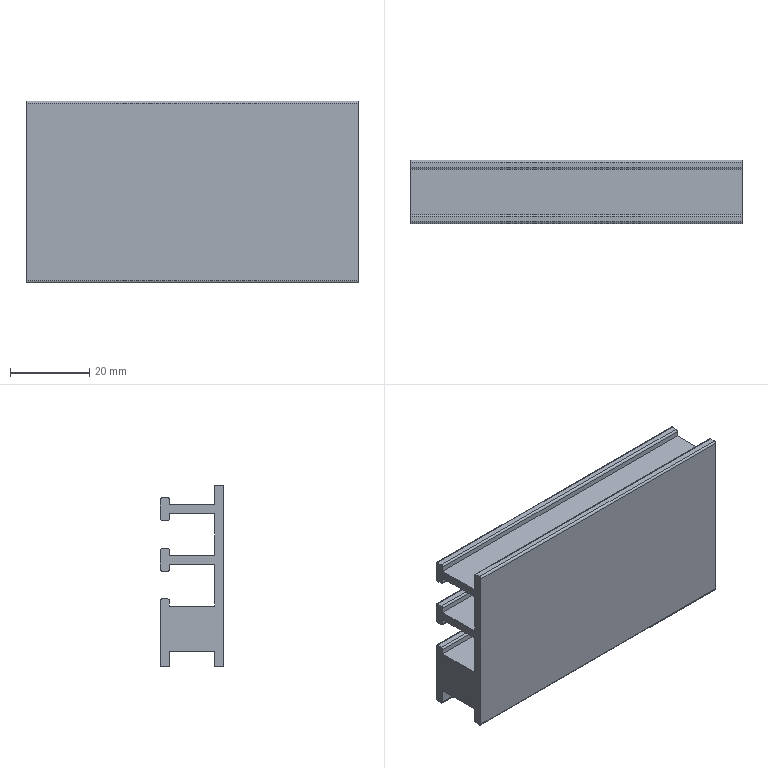Part | STEP file | Aluminium Alloy Bracket | 1 solid | 46 faces | box 84 x 16 x 46 mm | volume 29509 mm3 | plane 30 | cylinder 16 | commonest cylinder face diameters 1 x16
STEP:
#1=CARTESIAN_POINT('',(0.,0.,-0.5));
#2=VERTEX_POINT('',#1);
#3=CARTESIAN_POINT('',(84.,0.,-0.5));
#4=VERTEX_POINT('',#3);
#5=CARTESIAN_POINT('',(84.,0.,-0.5));
#6=DIRECTION('',(1.,0.,0.));
#7=VECTOR('',#6,1000.);
#8=LINE('',#5,#7);
#9=EDGE_CURVE('',#2,#4,#8,.T.);
#10=ORIENTED_EDGE('',*,*,#9,.F.);
#11=CARTESIAN_POINT('',(0.,0.,-45.5));
#12=VERTEX_POINT('',#11);
#13=CARTESIAN_POINT('',(0.,0.,-46.));
#14=DIRECTION('',(0.,0.,1.));
#15=VECTOR('',#14,1000.);
#16=LINE('',#13,#15);
#17=EDGE_CURVE('',#12,#2,#16,.T.);
#18=ORIENTED_EDGE('',*,*,#17,.F.);
#19=CARTESIAN_POINT('',(84.,0.,-45.5));
#20=VERTEX_POINT('',#19);
#21=CARTESIAN_POINT('',(84.,0.,-45.5));
#22=DIRECTION('',(-1.,0.,0.));
#23=VECTOR('',#22,1000.);
#24=LINE('',#21,#23);
#25=EDGE_CURVE('',#20,#12,#24,.T.);
#26=ORIENTED_EDGE('',*,*,#25,.F.);
#27=CARTESIAN_POINT('',(84.,0.,-46.));
#28=DIRECTION('',(0.,0.,-1.));
#29=VECTOR('',#28,1000.);
#30=LINE('',#27,#29);
#31=EDGE_CURVE('',#4,#20,#30,.T.);
#32=ORIENTED_EDGE('',*,*,#31,.F.);
#33=EDGE_LOOP('',(#10,#18,#26,#32));
#34=FACE_OUTER_BOUND('',#33,.T.);
#35=CARTESIAN_POINT('',(84.,0.,-46.));
#36=DIRECTION('',(0.,1.,0.));
#37=DIRECTION('',(0.,0.,1.));
#38=AXIS2_PLACEMENT_3D('',#35,#36,#37);
#39=PLANE('',#38);
#40=ADVANCED_FACE('',(#34),#39,.F.);
#41=CARTESIAN_POINT('',(84.,0.5,0.));
#42=VERTEX_POINT('',#41);
#43=CARTESIAN_POINT('',(84.,0.5,-0.5));
#44=DIRECTION('',(-1.,0.,0.));
#45=DIRECTION('',(0.,0.,1.));
#46=AXIS2_PLACEMENT_3D('',#43,#44,#45);
#47=CIRCLE('',#46,0.5);
#48=EDGE_CURVE('',#4,#42,#47,.T.);
#49=ORIENTED_EDGE('',*,*,#48,.F.);
#50=ORIENTED_EDGE('',*,*,#31,.T.);
#51=CARTESIAN_POINT('',(84.,0.5,-46.));
#52=VERTEX_POINT('',#51);
#53=CARTESIAN_POINT('',(84.,0.5,-45.5));
#54=DIRECTION('',(-1.,0.,0.));
#55=DIRECTION('',(0.,0.,1.));
#56=AXIS2_PLACEMENT_3D('',#53,#54,#55);
#57=CIRCLE('',#56,0.5);
#58=EDGE_CURVE('',#52,#20,#57,.T.);
#59=ORIENTED_EDGE('',*,*,#58,.F.);
#60=CARTESIAN_POINT('',(84.,1.8,-46.));
#61=VERTEX_POINT('',#60);
#62=CARTESIAN_POINT('',(84.,2.3,-46.));
#63=DIRECTION('',(0.,1.,0.));
#64=VECTOR('',#63,1000.);
#65=LINE('',#62,#64);
#66=EDGE_CURVE('',#52,#61,#65,.T.);
#67=ORIENTED_EDGE('',*,*,#66,.T.);
#68=CARTESIAN_POINT('',(84.,2.3,-45.5));
#69=VERTEX_POINT('',#68);
#70=CARTESIAN_POINT('',(84.,1.8,-45.5));
#71=DIRECTION('',(-1.,0.,0.));
#72=DIRECTION('',(0.,0.,1.));
#73=AXIS2_PLACEMENT_3D('',#70,#71,#72);
#74=CIRCLE('',#73,0.5);
#75=EDGE_CURVE('',#69,#61,#74,.T.);
#76=ORIENTED_EDGE('',*,*,#75,.F.);
#77=CARTESIAN_POINT('',(84.,2.3,-42.));
#78=VERTEX_POINT('',#77);
#79=CARTESIAN_POINT('',(84.,2.3,0.));
#80=DIRECTION('',(0.,0.,-1.));
#81=VECTOR('',#80,1000.);
#82=LINE('',#79,#81);
#83=EDGE_CURVE('',#78,#69,#82,.T.);
#84=ORIENTED_EDGE('',*,*,#83,.F.);
#85=CARTESIAN_POINT('',(84.,13.7,-42.));
#86=VERTEX_POINT('',#85);
#87=CARTESIAN_POINT('',(84.,0.,-42.));
#88=DIRECTION('',(0.,-1.,0.));
#89=VECTOR('',#88,1000.);
#90=LINE('',#87,#89);
#91=EDGE_CURVE('',#86,#78,#90,.T.);
#92=ORIENTED_EDGE('',*,*,#91,.F.);
#93=CARTESIAN_POINT('',(84.,13.7,-45.5));
#94=VERTEX_POINT('',#93);
#95=CARTESIAN_POINT('',(84.,13.7,0.));
#96=DIRECTION('',(0.,0.,1.));
#97=VECTOR('',#96,1000.);
#98=LINE('',#95,#97);
#99=EDGE_CURVE('',#94,#86,#98,.T.);
#100=ORIENTED_EDGE('',*,*,#99,.F.);
#101=CARTESIAN_POINT('',(84.,14.2,-46.));
#102=VERTEX_POINT('',#101);
#103=CARTESIAN_POINT('',(84.,14.2,-45.5));
#104=DIRECTION('',(-1.,0.,0.));
#105=DIRECTION('',(0.,0.,1.));
#106=AXIS2_PLACEMENT_3D('',#103,#104,#105);
#107=CIRCLE('',#106,0.5);
#108=EDGE_CURVE('',#102,#94,#107,.T.);
#109=ORIENTED_EDGE('',*,*,#108,.F.);
#110=CARTESIAN_POINT('',(84.,15.5,-46.));
#111=VERTEX_POINT('',#110);
#112=CARTESIAN_POINT('',(84.,16.,-46.));
#113=DIRECTION('',(0.,1.,0.));
#114=VECTOR('',#113,1000.);
#115=LINE('',#112,#114);
#116=EDGE_CURVE('',#102,#111,#115,.T.);
#117=ORIENTED_EDGE('',*,*,#116,.T.);
#118=CARTESIAN_POINT('',(84.,16.,-45.5));
#119=VERTEX_POINT('',#118);
#120=CARTESIAN_POINT('',(84.,15.5,-45.5));
#121=DIRECTION('',(-1.,0.,0.));
#122=DIRECTION('',(0.,0.,1.));
#123=AXIS2_PLACEMENT_3D('',#120,#121,#122);
#124=CIRCLE('',#123,0.5);
#125=EDGE_CURVE('',#119,#111,#124,.T.);
#126=ORIENTED_EDGE('',*,*,#125,.F.);
#127=CARTESIAN_POINT('',(84.,16.,-29.3));
#128=VERTEX_POINT('',#127);
#129=CARTESIAN_POINT('',(84.,16.,0.));
#130=DIRECTION('',(0.,0.,-1.));
#131=VECTOR('',#130,1000.);
#132=LINE('',#129,#131);
#133=EDGE_CURVE('',#128,#119,#132,.T.);
#134=ORIENTED_EDGE('',*,*,#133,.F.);
#135=CARTESIAN_POINT('',(84.,15.5,-28.8));
#136=VERTEX_POINT('',#135);
#137=CARTESIAN_POINT('',(84.,15.5,-29.3));
#138=DIRECTION('',(-1.,0.,0.));
#139=DIRECTION('',(0.,0.,1.));
#140=AXIS2_PLACEMENT_3D('',#137,#138,#139);
#141=CIRCLE('',#140,0.5);
#142=EDGE_CURVE('',#136,#128,#141,.T.);
#143=ORIENTED_EDGE('',*,*,#142,.F.);
#144=CARTESIAN_POINT('',(84.,14.2,-28.8));
#145=VERTEX_POINT('',#144);
#146=CARTESIAN_POINT('',(84.,13.7,-28.8));
#147=DIRECTION('',(0.,-1.,0.));
#148=VECTOR('',#147,1000.);
#149=LINE('',#146,#148);
#150=EDGE_CURVE('',#136,#145,#149,.T.);
#151=ORIENTED_EDGE('',*,*,#150,.T.);
#152=CARTESIAN_POINT('',(84.,13.7,-29.3));
#153=VERTEX_POINT('',#152);
#154=CARTESIAN_POINT('',(84.,14.2,-29.3));
#155=DIRECTION('',(-1.,0.,0.));
#156=DIRECTION('',(0.,0.,1.));
#157=AXIS2_PLACEMENT_3D('',#154,#155,#156);
#158=CIRCLE('',#157,0.5);
#159=EDGE_CURVE('',#153,#145,#158,.T.);
#160=ORIENTED_EDGE('',*,*,#159,.F.);
#161=CARTESIAN_POINT('',(84.,13.7,-30.6));
#162=VERTEX_POINT('',#161);
#163=CARTESIAN_POINT('',(84.,13.7,-30.6));
#164=DIRECTION('',(0.,0.,-1.));
#165=VECTOR('',#164,1000.);
#166=LINE('',#163,#165);
#167=EDGE_CURVE('',#153,#162,#166,.T.);
#168=ORIENTED_EDGE('',*,*,#167,.T.);
#169=CARTESIAN_POINT('',(84.,2.3,-30.6));
#170=VERTEX_POINT('',#169);
#171=CARTESIAN_POINT('',(84.,0.,-30.6));
#172=DIRECTION('',(0.,1.,0.));
#173=VECTOR('',#172,1000.);
#174=LINE('',#171,#173);
#175=EDGE_CURVE('',#170,#162,#174,.T.);
#176=ORIENTED_EDGE('',*,*,#175,.F.);
#177=CARTESIAN_POINT('',(84.,2.3,-20.));
#178=VERTEX_POINT('',#177);
#179=CARTESIAN_POINT('',(84.,2.3,0.));
#180=DIRECTION('',(0.,0.,-1.));
#181=VECTOR('',#180,1000.);
#182=LINE('',#179,#181);
#183=EDGE_CURVE('',#178,#170,#182,.T.);
#184=ORIENTED_EDGE('',*,*,#183,.F.);
#185=CARTESIAN_POINT('',(84.,13.7,-20.));
#186=VERTEX_POINT('',#185);
#187=CARTESIAN_POINT('',(84.,0.,-20.));
#188=DIRECTION('',(0.,-1.,0.));
#189=VECTOR('',#188,1000.);
#190=LINE('',#187,#189);
#191=EDGE_CURVE('',#186,#178,#190,.T.);
#192=ORIENTED_EDGE('',*,*,#191,.F.);
#193=CARTESIAN_POINT('',(84.,13.7,-21.3));
#194=VERTEX_POINT('',#193);
#195=CARTESIAN_POINT('',(84.,13.7,-21.8));
#196=DIRECTION('',(0.,0.,-1.));
#197=VECTOR('',#196,1000.);
#198=LINE('',#195,#197);
#199=EDGE_CURVE('',#186,#194,#198,.T.);
#200=ORIENTED_EDGE('',*,*,#199,.T.);
#201=CARTESIAN_POINT('',(84.,14.2,-21.8));
#202=VERTEX_POINT('',#201);
#203=CARTESIAN_POINT('',(84.,14.2,-21.3));
#204=DIRECTION('',(-1.,0.,0.));
#205=DIRECTION('',(0.,0.,1.));
#206=AXIS2_PLACEMENT_3D('',#203,#204,#205);
#207=CIRCLE('',#206,0.5);
#208=EDGE_CURVE('',#202,#194,#207,.T.);
#209=ORIENTED_EDGE('',*,*,#208,.F.);
#210=CARTESIAN_POINT('',(84.,15.5,-21.8));
#211=VERTEX_POINT('',#210);
#212=CARTESIAN_POINT('',(84.,16.,-21.8));
#213=DIRECTION('',(0.,1.,0.));
#214=VECTOR('',#213,1000.);
#215=LINE('',#212,#214);
#216=EDGE_CURVE('',#202,#211,#215,.T.);
#217=ORIENTED_EDGE('',*,*,#216,.T.);
#218=CARTESIAN_POINT('',(84.,16.,-21.3));
#219=VERTEX_POINT('',#218);
#220=CARTESIAN_POINT('',(84.,15.5,-21.3));
#221=DIRECTION('',(-1.,0.,0.));
#222=DIRECTION('',(0.,0.,1.));
#223=AXIS2_PLACEMENT_3D('',#220,#221,#222);
#224=CIRCLE('',#223,0.5);
#225=EDGE_CURVE('',#219,#211,#224,.T.);
#226=ORIENTED_EDGE('',*,*,#225,.F.);
#227=CARTESIAN_POINT('',(84.,16.,-16.5));
#228=VERTEX_POINT('',#227);
#229=CARTESIAN_POINT('',(84.,16.,0.));
#230=DIRECTION('',(0.,0.,-1.));
#231=VECTOR('',#230,1000.);
#232=LINE('',#229,#231);
#233=EDGE_CURVE('',#228,#219,#232,.T.);
#234=ORIENTED_EDGE('',*,*,#233,.F.);
#235=CARTESIAN_POINT('',(84.,15.5,-16.));
#236=VERTEX_POINT('',#235);
#237=CARTESIAN_POINT('',(84.,15.5,-16.5));
#238=DIRECTION('',(-1.,0.,0.));
#239=DIRECTION('',(0.,0.,1.));
#240=AXIS2_PLACEMENT_3D('',#237,#238,#239);
#241=CIRCLE('',#240,0.5);
#242=EDGE_CURVE('',#236,#228,#241,.T.);
#243=ORIENTED_EDGE('',*,*,#242,.F.);
#244=CARTESIAN_POINT('',(84.,14.2,-16.));
#245=VERTEX_POINT('',#244);
#246=CARTESIAN_POINT('',(84.,13.7,-16.));
#247=DIRECTION('',(0.,-1.,0.));
#248=VECTOR('',#247,1000.);
#249=LINE('',#246,#248);
#250=EDGE_CURVE('',#236,#245,#249,.T.);
#251=ORIENTED_EDGE('',*,*,#250,.T.);
#252=CARTESIAN_POINT('',(84.,13.7,-16.5));
#253=VERTEX_POINT('',#252);
#254=CARTESIAN_POINT('',(84.,14.2,-16.5));
#255=DIRECTION('',(-1.,0.,0.));
#256=DIRECTION('',(0.,0.,1.));
#257=AXIS2_PLACEMENT_3D('',#254,#255,#256);
#258=CIRCLE('',#257,0.5);
#259=EDGE_CURVE('',#253,#245,#258,.T.);
#260=ORIENTED_EDGE('',*,*,#259,.F.);
#261=CARTESIAN_POINT('',(84.,13.7,-17.8));
#262=VERTEX_POINT('',#261);
#263=CARTESIAN_POINT('',(84.,13.7,-17.8));
#264=DIRECTION('',(0.,0.,-1.));
#265=VECTOR('',#264,1000.);
#266=LINE('',#263,#265);
#267=EDGE_CURVE('',#253,#262,#266,.T.);
#268=ORIENTED_EDGE('',*,*,#267,.T.);
#269=CARTESIAN_POINT('',(84.,2.3,-17.8));
#270=VERTEX_POINT('',#269);
#271=CARTESIAN_POINT('',(84.,0.,-17.8));
#272=DIRECTION('',(0.,1.,0.));
#273=VECTOR('',#272,1000.);
#274=LINE('',#271,#273);
#275=EDGE_CURVE('',#270,#262,#274,.T.);
#276=ORIENTED_EDGE('',*,*,#275,.F.);
#277=CARTESIAN_POINT('',(84.,2.3,-7.2));
#278=VERTEX_POINT('',#277);
#279=CARTESIAN_POINT('',(84.,2.3,0.));
#280=DIRECTION('',(0.,0.,-1.));
#281=VECTOR('',#280,1000.);
#282=LINE('',#279,#281);
#283=EDGE_CURVE('',#278,#270,#282,.T.);
#284=ORIENTED_EDGE('',*,*,#283,.F.);
#285=CARTESIAN_POINT('',(84.,13.7,-7.2));
#286=VERTEX_POINT('',#285);
#287=CARTESIAN_POINT('',(84.,0.,-7.2));
#288=DIRECTION('',(0.,-1.,0.));
#289=VECTOR('',#288,1000.);
#290=LINE('',#287,#289);
#291=EDGE_CURVE('',#286,#278,#290,.T.);
#292=ORIENTED_EDGE('',*,*,#291,.F.);
#293=CARTESIAN_POINT('',(84.,13.7,-8.5));
#294=VERTEX_POINT('',#293);
#295=CARTESIAN_POINT('',(84.,13.7,-9.));
#296=DIRECTION('',(0.,0.,-1.));
#297=VECTOR('',#296,1000.);
#298=LINE('',#295,#297);
#299=EDGE_CURVE('',#286,#294,#298,.T.);
#300=ORIENTED_EDGE('',*,*,#299,.T.);
#301=CARTESIAN_POINT('',(84.,14.2,-9.));
#302=VERTEX_POINT('',#301);
#303=CARTESIAN_POINT('',(84.,14.2,-8.5));
#304=DIRECTION('',(-1.,0.,0.));
#305=DIRECTION('',(0.,0.,1.));
#306=AXIS2_PLACEMENT_3D('',#303,#304,#305);
#307=CIRCLE('',#306,0.5);
#308=EDGE_CURVE('',#302,#294,#307,.T.);
#309=ORIENTED_EDGE('',*,*,#308,.F.);
#310=CARTESIAN_POINT('',(84.,15.5,-9.));
#311=VERTEX_POINT('',#310);
#312=CARTESIAN_POINT('',(84.,16.,-9.));
#313=DIRECTION('',(0.,1.,0.));
#314=VECTOR('',#313,1000.);
#315=LINE('',#312,#314);
#316=EDGE_CURVE('',#302,#311,#315,.T.);
#317=ORIENTED_EDGE('',*,*,#316,.T.);
#318=CARTESIAN_POINT('',(84.,16.,-8.5));
#319=VERTEX_POINT('',#318);
#320=CARTESIAN_POINT('',(84.,15.5,-8.5));
#321=DIRECTION('',(-1.,0.,0.));
#322=DIRECTION('',(0.,0.,1.));
#323=AXIS2_PLACEMENT_3D('',#320,#321,#322);
#324=CIRCLE('',#323,0.5);
#325=EDGE_CURVE('',#319,#311,#324,.T.);
#326=ORIENTED_EDGE('',*,*,#325,.F.);
#327=CARTESIAN_POINT('',(84.,16.,-3.7));
#328=VERTEX_POINT('',#327);
#329=CARTESIAN_POINT('',(84.,16.,0.));
#330=DIRECTION('',(0.,0.,-1.));
#331=VECTOR('',#330,1000.);
#332=LINE('',#329,#331);
#333=EDGE_CURVE('',#328,#319,#332,.T.);
#334=ORIENTED_EDGE('',*,*,#333,.F.);
#335=CARTESIAN_POINT('',(84.,15.5,-3.2));
#336=VERTEX_POINT('',#335);
#337=CARTESIAN_POINT('',(84.,15.5,-3.7));
#338=DIRECTION('',(-1.,0.,0.));
#339=DIRECTION('',(0.,0.,1.));
#340=AXIS2_PLACEMENT_3D('',#337,#338,#339);
#341=CIRCLE('',#340,0.5);
#342=EDGE_CURVE('',#336,#328,#341,.T.);
#343=ORIENTED_EDGE('',*,*,#342,.F.);
#344=CARTESIAN_POINT('',(84.,14.2,-3.2));
#345=VERTEX_POINT('',#344);
#346=CARTESIAN_POINT('',(84.,13.7,-3.2));
#347=DIRECTION('',(0.,-1.,0.));
#348=VECTOR('',#347,1000.);
#349=LINE('',#346,#348);
#350=EDGE_CURVE('',#336,#345,#349,.T.);
#351=ORIENTED_EDGE('',*,*,#350,.T.);
#352=CARTESIAN_POINT('',(84.,13.7,-3.7));
#353=VERTEX_POINT('',#352);
#354=CARTESIAN_POINT('',(84.,14.2,-3.7));
#355=DIRECTION('',(-1.,0.,0.));
#356=DIRECTION('',(0.,0.,1.));
#357=AXIS2_PLACEMENT_3D('',#354,#355,#356);
#358=CIRCLE('',#357,0.5);
#359=EDGE_CURVE('',#353,#345,#358,.T.);
#360=ORIENTED_EDGE('',*,*,#359,.F.);
#361=CARTESIAN_POINT('',(84.,13.7,-5.));
#362=VERTEX_POINT('',#361);
#363=CARTESIAN_POINT('',(84.,13.7,-5.));
#364=DIRECTION('',(0.,0.,-1.));
#365=VECTOR('',#364,1000.);
#366=LINE('',#363,#365);
#367=EDGE_CURVE('',#353,#362,#366,.T.);
#368=ORIENTED_EDGE('',*,*,#367,.T.);
#369=CARTESIAN_POINT('',(84.,2.3,-5.));
#370=VERTEX_POINT('',#369);
#371=CARTESIAN_POINT('',(84.,0.,-5.));
#372=DIRECTION('',(0.,1.,0.));
#373=VECTOR('',#372,1000.);
#374=LINE('',#371,#373);
#375=EDGE_CURVE('',#370,#362,#374,.T.);
#376=ORIENTED_EDGE('',*,*,#375,.F.);
#377=CARTESIAN_POINT('',(84.,2.3,-0.5));
#378=VERTEX_POINT('',#377);
#379=CARTESIAN_POINT('',(84.,2.3,0.));
#380=DIRECTION('',(0.,0.,-1.));
#381=VECTOR('',#380,1000.);
#382=LINE('',#379,#381);
#383=EDGE_CURVE('',#378,#370,#382,.T.);
#384=ORIENTED_EDGE('',*,*,#383,.F.);
#385=CARTESIAN_POINT('',(84.,1.8,0.));
#386=VERTEX_POINT('',#385);
#387=CARTESIAN_POINT('',(84.,1.8,-0.5));
#388=DIRECTION('',(-1.,0.,0.));
#389=DIRECTION('',(0.,0.,1.));
#390=AXIS2_PLACEMENT_3D('',#387,#388,#389);
#391=CIRCLE('',#390,0.5);
#392=EDGE_CURVE('',#386,#378,#391,.T.);
#393=ORIENTED_EDGE('',*,*,#392,.F.);
#394=CARTESIAN_POINT('',(84.,0.,0.));
#395=DIRECTION('',(0.,-1.,0.));
#396=VECTOR('',#395,1000.);
#397=LINE('',#394,#396);
#398=EDGE_CURVE('',#386,#42,#397,.T.);
#399=ORIENTED_EDGE('',*,*,#398,.T.);
#400=EDGE_LOOP('',(#49,#50,#59,#67,#76,#84,#92,#100,#109,#117,#126,#134,#143,#151,#160,#168,#176,#184,#192,#200,#209,#217,#226,#234,#243,#251,#260,#268,#276,#284,#292,#300,#309,#317,#326,#334,#343,#351,#360,#368,#376,#384,#393,#399));
#401=FACE_OUTER_BOUND('',#400,.T.);
#402=CARTESIAN_POINT('',(84.,0.,0.));
#403=DIRECTION('',(-1.,0.,0.));
#404=DIRECTION('',(0.,0.,1.));
#405=AXIS2_PLACEMENT_3D('',#402,#403,#404);
#406=PLANE('',#405);
#407=ADVANCED_FACE('',(#401),#406,.F.);
#408=CARTESIAN_POINT('',(0.,0.5,0.));
#409=VERTEX_POINT('',#408);
#410=CARTESIAN_POINT('',(0.,0.5,-0.5));
#411=DIRECTION('',(1.,0.,0.));
#412=DIRECTION('',(0.,0.,1.));
#413=AXIS2_PLACEMENT_3D('',#410,#411,#412);
#414=CIRCLE('',#413,0.5);
#415=EDGE_CURVE('',#409,#2,#414,.T.);
#416=ORIENTED_EDGE('',*,*,#415,.T.);
#417=ORIENTED_EDGE('',*,*,#9,.T.);
#418=ORIENTED_EDGE('',*,*,#48,.T.);
#419=CARTESIAN_POINT('',(84.,0.5,0.));
#420=DIRECTION('',(-1.,0.,0.));
#421=VECTOR('',#420,1000.);
#422=LINE('',#419,#421);
#423=EDGE_CURVE('',#42,#409,#422,.T.);
#424=ORIENTED_EDGE('',*,*,#423,.T.);
#425=EDGE_LOOP('',(#416,#417,#418,#424));
#426=FACE_OUTER_BOUND('',#425,.T.);
#427=CARTESIAN_POINT('',(84.,0.5,-0.5));
#428=DIRECTION('',(-1.,0.,0.));
#429=DIRECTION('',(0.,0.,1.));
#430=AXIS2_PLACEMENT_3D('',#427,#428,#429);
#431=CYLINDRICAL_SURFACE('',#430,0.5);
#432=ADVANCED_FACE('',(#426),#431,.T.);
#433=CARTESIAN_POINT('',(0.,1.8,-46.));
#434=VERTEX_POINT('',#433);
#435=CARTESIAN_POINT('',(0.,0.5,-46.));
#436=VERTEX_POINT('',#435);
#437=CARTESIAN_POINT('',(0.,2.3,-46.));
#438=DIRECTION('',(0.,-1.,0.));
#439=VECTOR('',#438,1000.);
#440=LINE('',#437,#439);
#441=EDGE_CURVE('',#434,#436,#440,.T.);
#442=ORIENTED_EDGE('',*,*,#441,.T.);
#443=CARTESIAN_POINT('',(0.,0.5,-45.5));
#444=DIRECTION('',(-1.,0.,0.));
#445=DIRECTION('',(0.,0.,1.));
#446=AXIS2_PLACEMENT_3D('',#443,#444,#445);
#447=CIRCLE('',#446,0.5);
#448=EDGE_CURVE('',#436,#12,#447,.T.);
#449=ORIENTED_EDGE('',*,*,#448,.T.);
#450=ORIENTED_EDGE('',*,*,#17,.T.);
#451=ORIENTED_EDGE('',*,*,#415,.F.);
#452=CARTESIAN_POINT('',(0.,1.8,0.));
#453=VERTEX_POINT('',#452);
#454=CARTESIAN_POINT('',(0.,0.,0.));
#455=DIRECTION('',(0.,1.,0.));
#456=VECTOR('',#455,1000.);
#457=LINE('',#454,#456);
#458=EDGE_CURVE('',#409,#453,#457,.T.);
#459=ORIENTED_EDGE('',*,*,#458,.T.);
#460=CARTESIAN_POINT('',(0.,2.3,-0.5));
#461=VERTEX_POINT('',#460);
#462=CARTESIAN_POINT('',(0.,1.8,-0.5));
#463=DIRECTION('',(1.,0.,0.));
#464=DIRECTION('',(0.,0.,1.));
#465=AXIS2_PLACEMENT_3D('',#462,#463,#464);
#466=CIRCLE('',#465,0.5);
#467=EDGE_CURVE('',#461,#453,#466,.T.);
#468=ORIENTED_EDGE('',*,*,#467,.F.);
#469=CARTESIAN_POINT('',(0.,2.3,-5.));
#470=VERTEX_POINT('',#469);
#471=CARTESIAN_POINT('',(0.,2.3,0.));
#472=DIRECTION('',(0.,0.,-1.));
#473=VECTOR('',#472,1000.);
#474=LINE('',#471,#473);
#475=EDGE_CURVE('',#461,#470,#474,.T.);
#476=ORIENTED_EDGE('',*,*,#475,.T.);
#477=CARTESIAN_POINT('',(0.,13.7,-5.));
#478=VERTEX_POINT('',#477);
#479=CARTESIAN_POINT('',(0.,0.,-5.));
#480=DIRECTION('',(0.,1.,0.));
#481=VECTOR('',#480,1000.);
#482=LINE('',#479,#481);
#483=EDGE_CURVE('',#470,#478,#482,.T.);
#484=ORIENTED_EDGE('',*,*,#483,.T.);
#485=CARTESIAN_POINT('',(0.,13.7,-3.7));
#486=VERTEX_POINT('',#485);
#487=CARTESIAN_POINT('',(0.,13.7,-5.));
#488=DIRECTION('',(0.,0.,1.));
#489=VECTOR('',#488,1000.);
#490=LINE('',#487,#489);
#491=EDGE_CURVE('',#478,#486,#490,.T.);
#492=ORIENTED_EDGE('',*,*,#491,.T.);
#493=CARTESIAN_POINT('',(0.,14.2,-3.2));
#494=VERTEX_POINT('',#493);
#495=CARTESIAN_POINT('',(0.,14.2,-3.7));
#496=DIRECTION('',(1.,0.,0.));
#497=DIRECTION('',(0.,0.,1.));
#498=AXIS2_PLACEMENT_3D('',#495,#496,#497);
#499=CIRCLE('',#498,0.5);
#500=EDGE_CURVE('',#494,#486,#499,.T.);
#501=ORIENTED_EDGE('',*,*,#500,.F.);
#502=CARTESIAN_POINT('',(0.,15.5,-3.2));
#503=VERTEX_POINT('',#502);
#504=CARTESIAN_POINT('',(0.,13.7,-3.2));
#505=DIRECTION('',(0.,1.,0.));
#506=VECTOR('',#505,1000.);
#507=LINE('',#504,#506);
#508=EDGE_CURVE('',#494,#503,#507,.T.);
#509=ORIENTED_EDGE('',*,*,#508,.T.);
#510=CARTESIAN_POINT('',(0.,16.,-3.7));
#511=VERTEX_POINT('',#510);
#512=CARTESIAN_POINT('',(0.,15.5,-3.7));
#513=DIRECTION('',(1.,0.,0.));
#514=DIRECTION('',(0.,0.,1.));
#515=AXIS2_PLACEMENT_3D('',#512,#513,#514);
#516=CIRCLE('',#515,0.5);
#517=EDGE_CURVE('',#511,#503,#516,.T.);
#518=ORIENTED_EDGE('',*,*,#517,.F.);
#519=CARTESIAN_POINT('',(0.,16.,-8.5));
#520=VERTEX_POINT('',#519);
#521=CARTESIAN_POINT('',(0.,16.,0.));
#522=DIRECTION('',(0.,0.,-1.));
#523=VECTOR('',#522,1000.);
#524=LINE('',#521,#523);
#525=EDGE_CURVE('',#511,#520,#524,.T.);
#526=ORIENTED_EDGE('',*,*,#525,.T.);
#527=CARTESIAN_POINT('',(0.,15.5,-9.));
#528=VERTEX_POINT('',#527);
#529=CARTESIAN_POINT('',(0.,15.5,-8.5));
#530=DIRECTION('',(1.,0.,0.));
#531=DIRECTION('',(0.,0.,1.));
#532=AXIS2_PLACEMENT_3D('',#529,#530,#531);
#533=CIRCLE('',#532,0.5);
#534=EDGE_CURVE('',#528,#520,#533,.T.);
#535=ORIENTED_EDGE('',*,*,#534,.F.);
#536=CARTESIAN_POINT('',(0.,14.2,-9.));
#537=VERTEX_POINT('',#536);
#538=CARTESIAN_POINT('',(0.,16.,-9.));
#539=DIRECTION('',(0.,-1.,0.));
#540=VECTOR('',#539,1000.);
#541=LINE('',#538,#540);
#542=EDGE_CURVE('',#528,#537,#541,.T.);
#543=ORIENTED_EDGE('',*,*,#542,.T.);
#544=CARTESIAN_POINT('',(0.,13.7,-8.5));
#545=VERTEX_POINT('',#544);
#546=CARTESIAN_POINT('',(0.,14.2,-8.5));
#547=DIRECTION('',(1.,0.,0.));
#548=DIRECTION('',(0.,0.,1.));
#549=AXIS2_PLACEMENT_3D('',#546,#547,#548);
#550=CIRCLE('',#549,0.5);
#551=EDGE_CURVE('',#545,#537,#550,.T.);
#552=ORIENTED_EDGE('',*,*,#551,.F.);
#553=CARTESIAN_POINT('',(0.,13.7,-7.2));
#554=VERTEX_POINT('',#553);
#555=CARTESIAN_POINT('',(0.,13.7,-9.));
#556=DIRECTION('',(0.,0.,1.));
#557=VECTOR('',#556,1000.);
#558=LINE('',#555,#557);
#559=EDGE_CURVE('',#545,#554,#558,.T.);
#560=ORIENTED_EDGE('',*,*,#559,.T.);
#561=CARTESIAN_POINT('',(0.,2.3,-7.2));
#562=VERTEX_POINT('',#561);
#563=CARTESIAN_POINT('',(0.,0.,-7.2));
#564=DIRECTION('',(0.,-1.,0.));
#565=VECTOR('',#564,1000.);
#566=LINE('',#563,#565);
#567=EDGE_CURVE('',#554,#562,#566,.T.);
#568=ORIENTED_EDGE('',*,*,#567,.T.);
#569=CARTESIAN_POINT('',(0.,2.3,-17.8));
#570=VERTEX_POINT('',#569);
#571=CARTESIAN_POINT('',(0.,2.3,0.));
#572=DIRECTION('',(0.,0.,-1.));
#573=VECTOR('',#572,1000.);
#574=LINE('',#571,#573);
#575=EDGE_CURVE('',#562,#570,#574,.T.);
#576=ORIENTED_EDGE('',*,*,#575,.T.);
#577=CARTESIAN_POINT('',(0.,13.7,-17.8));
#578=VERTEX_POINT('',#577);
#579=CARTESIAN_POINT('',(0.,0.,-17.8));
#580=DIRECTION('',(0.,1.,0.));
#581=VECTOR('',#580,1000.);
#582=LINE('',#579,#581);
#583=EDGE_CURVE('',#570,#578,#582,.T.);
#584=ORIENTED_EDGE('',*,*,#583,.T.);
#585=CARTESIAN_POINT('',(0.,13.7,-16.5));
#586=VERTEX_POINT('',#585);
#587=CARTESIAN_POINT('',(0.,13.7,-17.8));
#588=DIRECTION('',(0.,0.,1.));
#589=VECTOR('',#588,1000.);
#590=LINE('',#587,#589);
#591=EDGE_CURVE('',#578,#586,#590,.T.);
#592=ORIENTED_EDGE('',*,*,#591,.T.);
#593=CARTESIAN_POINT('',(0.,14.2,-16.));
#594=VERTEX_POINT('',#593);
#595=CARTESIAN_POINT('',(0.,14.2,-16.5));
#596=DIRECTION('',(1.,0.,0.));
#597=DIRECTION('',(0.,0.,1.));
#598=AXIS2_PLACEMENT_3D('',#595,#596,#597);
#599=CIRCLE('',#598,0.5);
#600=EDGE_CURVE('',#594,#586,#599,.T.);
#601=ORIENTED_EDGE('',*,*,#600,.F.);
#602=CARTESIAN_POINT('',(0.,15.5,-16.));
#603=VERTEX_POINT('',#602);
#604=CARTESIAN_POINT('',(0.,13.7,-16.));
#605=DIRECTION('',(0.,1.,0.));
#606=VECTOR('',#605,1000.);
#607=LINE('',#604,#606);
#608=EDGE_CURVE('',#594,#603,#607,.T.);
#609=ORIENTED_EDGE('',*,*,#608,.T.);
#610=CARTESIAN_POINT('',(0.,16.,-16.5));
#611=VERTEX_POINT('',#610);
#612=CARTESIAN_POINT('',(0.,15.5,-16.5));
#613=DIRECTION('',(1.,0.,0.));
#614=DIRECTION('',(0.,0.,1.));
#615=AXIS2_PLACEMENT_3D('',#612,#613,#614);
#616=CIRCLE('',#615,0.5);
#617=EDGE_CURVE('',#611,#603,#616,.T.);
#618=ORIENTED_EDGE('',*,*,#617,.F.);
#619=CARTESIAN_POINT('',(0.,16.,-21.3));
#620=VERTEX_POINT('',#619);
#621=CARTESIAN_POINT('',(0.,16.,0.));
#622=DIRECTION('',(0.,0.,-1.));
#623=VECTOR('',#622,1000.);
#624=LINE('',#621,#623);
#625=EDGE_CURVE('',#611,#620,#624,.T.);
#626=ORIENTED_EDGE('',*,*,#625,.T.);
#627=CARTESIAN_POINT('',(0.,15.5,-21.8));
#628=VERTEX_POINT('',#627);
#629=CARTESIAN_POINT('',(0.,15.5,-21.3));
#630=DIRECTION('',(1.,0.,0.));
#631=DIRECTION('',(0.,0.,1.));
#632=AXIS2_PLACEMENT_3D('',#629,#630,#631);
#633=CIRCLE('',#632,0.5);
#634=EDGE_CURVE('',#628,#620,#633,.T.);
#635=ORIENTED_EDGE('',*,*,#634,.F.);
#636=CARTESIAN_POINT('',(0.,14.2,-21.8));
#637=VERTEX_POINT('',#636);
#638=CARTESIAN_POINT('',(0.,16.,-21.8));
#639=DIRECTION('',(0.,-1.,0.));
#640=VECTOR('',#639,1000.);
#641=LINE('',#638,#640);
#642=EDGE_CURVE('',#628,#637,#641,.T.);
#643=ORIENTED_EDGE('',*,*,#642,.T.);
#644=CARTESIAN_POINT('',(0.,13.7,-21.3));
#645=VERTEX_POINT('',#644);
#646=CARTESIAN_POINT('',(0.,14.2,-21.3));
#647=DIRECTION('',(1.,0.,0.));
#648=DIRECTION('',(0.,0.,1.));
#649=AXIS2_PLACEMENT_3D('',#646,#647,#648);
#650=CIRCLE('',#649,0.5);
#651=EDGE_CURVE('',#645,#637,#650,.T.);
#652=ORIENTED_EDGE('',*,*,#651,.F.);
#653=CARTESIAN_POINT('',(0.,13.7,-20.));
#654=VERTEX_POINT('',#653);
#655=CARTESIAN_POINT('',(0.,13.7,-21.8));
#656=DIRECTION('',(0.,0.,1.));
#657=VECTOR('',#656,1000.);
#658=LINE('',#655,#657);
#659=EDGE_CURVE('',#645,#654,#658,.T.);
#660=ORIENTED_EDGE('',*,*,#659,.T.);
#661=CARTESIAN_POINT('',(0.,2.3,-20.));
#662=VERTEX_POINT('',#661);
#663=CARTESIAN_POINT('',(0.,0.,-20.));
#664=DIRECTION('',(0.,-1.,0.));
#665=VECTOR('',#664,1000.);
#666=LINE('',#663,#665);
#667=EDGE_CURVE('',#654,#662,#666,.T.);
#668=ORIENTED_EDGE('',*,*,#667,.T.);
#669=CARTESIAN_POINT('',(0.,2.3,-30.6));
#670=VERTEX_POINT('',#669);
#671=CARTESIAN_POINT('',(0.,2.3,0.));
#672=DIRECTION('',(0.,0.,-1.));
#673=VECTOR('',#672,1000.);
#674=LINE('',#671,#673);
#675=EDGE_CURVE('',#662,#670,#674,.T.);
#676=ORIENTED_EDGE('',*,*,#675,.T.);
#677=CARTESIAN_POINT('',(0.,13.7,-30.6));
#678=VERTEX_POINT('',#677);
#679=CARTESIAN_POINT('',(0.,0.,-30.6));
#680=DIRECTION('',(0.,1.,0.));
#681=VECTOR('',#680,1000.);
#682=LINE('',#679,#681);
#683=EDGE_CURVE('',#670,#678,#682,.T.);
#684=ORIENTED_EDGE('',*,*,#683,.T.);
#685=CARTESIAN_POINT('',(0.,13.7,-29.3));
#686=VERTEX_POINT('',#685);
#687=CARTESIAN_POINT('',(0.,13.7,-30.6));
#688=DIRECTION('',(0.,0.,1.));
#689=VECTOR('',#688,1000.);
#690=LINE('',#687,#689);
#691=EDGE_CURVE('',#678,#686,#690,.T.);
#692=ORIENTED_EDGE('',*,*,#691,.T.);
#693=CARTESIAN_POINT('',(0.,14.2,-28.8));
#694=VERTEX_POINT('',#693);
#695=CARTESIAN_POINT('',(0.,14.2,-29.3));
#696=DIRECTION('',(1.,0.,0.));
#697=DIRECTION('',(0.,0.,1.));
#698=AXIS2_PLACEMENT_3D('',#695,#696,#697);
#699=CIRCLE('',#698,0.5);
#700=EDGE_CURVE('',#694,#686,#699,.T.);
#701=ORIENTED_EDGE('',*,*,#700,.F.);
#702=CARTESIAN_POINT('',(0.,15.5,-28.8));
#703=VERTEX_POINT('',#702);
#704=CARTESIAN_POINT('',(0.,13.7,-28.8));
#705=DIRECTION('',(0.,1.,0.));
#706=VECTOR('',#705,1000.);
#707=LINE('',#704,#706);
#708=EDGE_CURVE('',#694,#703,#707,.T.);
#709=ORIENTED_EDGE('',*,*,#708,.T.);
#710=CARTESIAN_POINT('',(0.,16.,-29.3));
#711=VERTEX_POINT('',#710);
#712=CARTESIAN_POINT('',(0.,15.5,-29.3));
#713=DIRECTION('',(1.,0.,0.));
#714=DIRECTION('',(0.,0.,1.));
#715=AXIS2_PLACEMENT_3D('',#712,#713,#714);
#716=CIRCLE('',#715,0.5);
#717=EDGE_CURVE('',#711,#703,#716,.T.);
#718=ORIENTED_EDGE('',*,*,#717,.F.);
#719=CARTESIAN_POINT('',(0.,16.,-45.5));
#720=VERTEX_POINT('',#719);
#721=CARTESIAN_POINT('',(0.,16.,0.));
#722=DIRECTION('',(0.,0.,-1.));
#723=VECTOR('',#722,1000.);
#724=LINE('',#721,#723);
#725=EDGE_CURVE('',#711,#720,#724,.T.);
#726=ORIENTED_EDGE('',*,*,#725,.T.);
#727=CARTESIAN_POINT('',(0.,15.5,-46.));
#728=VERTEX_POINT('',#727);
#729=CARTESIAN_POINT('',(0.,15.5,-45.5));
#730=DIRECTION('',(1.,0.,0.));
#731=DIRECTION('',(0.,0.,1.));
#732=AXIS2_PLACEMENT_3D('',#729,#730,#731);
#733=CIRCLE('',#732,0.5);
#734=EDGE_CURVE('',#728,#720,#733,.T.);
#735=ORIENTED_EDGE('',*,*,#734,.F.);
#736=CARTESIAN_POINT('',(0.,14.2,-46.));
#737=VERTEX_POINT('',#736);
#738=CARTESIAN_POINT('',(0.,16.,-46.));
#739=DIRECTION('',(0.,-1.,0.));
#740=VECTOR('',#739,1000.);
#741=LINE('',#738,#740);
#742=EDGE_CURVE('',#728,#737,#741,.T.);
#743=ORIENTED_EDGE('',*,*,#742,.T.);
#744=CARTESIAN_POINT('',(0.,13.7,-45.5));
#745=VERTEX_POINT('',#744);
#746=CARTESIAN_POINT('',(0.,14.2,-45.5));
#747=DIRECTION('',(1.,0.,0.));
#748=DIRECTION('',(0.,0.,1.));
#749=AXIS2_PLACEMENT_3D('',#746,#747,#748);
#750=CIRCLE('',#749,0.5);
#751=EDGE_CURVE('',#745,#737,#750,.T.);
#752=ORIENTED_EDGE('',*,*,#751,.F.);
#753=CARTESIAN_POINT('',(0.,13.7,-42.));
#754=VERTEX_POINT('',#753);
#755=CARTESIAN_POINT('',(0.,13.7,0.));
#756=DIRECTION('',(0.,0.,1.));
#757=VECTOR('',#756,1000.);
#758=LINE('',#755,#757);
#759=EDGE_CURVE('',#745,#754,#758,.T.);
#760=ORIENTED_EDGE('',*,*,#759,.T.);
#761=CARTESIAN_POINT('',(0.,2.3,-42.));
#762=VERTEX_POINT('',#761);
#763=CARTESIAN_POINT('',(0.,0.,-42.));
#764=DIRECTION('',(0.,-1.,0.));
#765=VECTOR('',#764,1000.);
#766=LINE('',#763,#765);
#767=EDGE_CURVE('',#754,#762,#766,.T.);
#768=ORIENTED_EDGE('',*,*,#767,.T.);
#769=CARTESIAN_POINT('',(0.,2.3,-45.5));
#770=VERTEX_POINT('',#769);
#771=CARTESIAN_POINT('',(0.,2.3,0.));
#772=DIRECTION('',(0.,0.,-1.));
#773=VECTOR('',#772,1000.);
#774=LINE('',#771,#773);
#775=EDGE_CURVE('',#762,#770,#774,.T.);
#776=ORIENTED_EDGE('',*,*,#775,.T.);
#777=CARTESIAN_POINT('',(0.,1.8,-45.5));
#778=DIRECTION('',(1.,0.,0.));
#779=DIRECTION('',(0.,0.,1.));
#780=AXIS2_PLACEMENT_3D('',#777,#778,#779);
#781=CIRCLE('',#780,0.5);
#782=EDGE_CURVE('',#434,#770,#781,.T.);
#783=ORIENTED_EDGE('',*,*,#782,.F.);
#784=EDGE_LOOP('',(#442,#449,#450,#451,#459,#468,#476,#484,#492,#501,#509,#518,#526,#535,#543,#552,#560,#568,#576,#584,#592,#601,#609,#618,#626,#635,#643,#652,#660,#668,#676,#684,#692,#701,#709,#718,#726,#735,#743,#752,#760,#768,#776,#783));
#785=FACE_OUTER_BOUND('',#784,.T.);
#786=CARTESIAN_POINT('',(0.,0.,0.));
#787=DIRECTION('',(-1.,0.,0.));
#788=DIRECTION('',(0.,0.,1.));
#789=AXIS2_PLACEMENT_3D('',#786,#787,#788);
#790=PLANE('',#789);
#791=ADVANCED_FACE('',(#785),#790,.T.);
#792=ORIENTED_EDGE('',*,*,#448,.F.);
#793=CARTESIAN_POINT('',(84.,0.5,-46.));
#794=DIRECTION('',(1.,0.,0.));
#795=VECTOR('',#794,1000.);
#796=LINE('',#793,#795);
#797=EDGE_CURVE('',#436,#52,#796,.T.);
#798=ORIENTED_EDGE('',*,*,#797,.T.);
#799=ORIENTED_EDGE('',*,*,#58,.T.);
#800=ORIENTED_EDGE('',*,*,#25,.T.);
#801=EDGE_LOOP('',(#792,#798,#799,#800));
#802=FACE_OUTER_BOUND('',#801,.T.);
#803=CARTESIAN_POINT('',(84.,0.5,-45.5));
#804=DIRECTION('',(-1.,0.,0.));
#805=DIRECTION('',(0.,0.,1.));
#806=AXIS2_PLACEMENT_3D('',#803,#804,#805);
#807=CYLINDRICAL_SURFACE('',#806,0.5);
#808=ADVANCED_FACE('',(#802),#807,.T.);
#809=CARTESIAN_POINT('',(84.,2.3,-45.5));
#810=DIRECTION('',(1.,0.,0.));
#811=VECTOR('',#810,1000.);
#812=LINE('',#809,#811);
#813=EDGE_CURVE('',#770,#69,#812,.T.);
#814=ORIENTED_EDGE('',*,*,#813,.F.);
#815=ORIENTED_EDGE('',*,*,#775,.F.);
#816=CARTESIAN_POINT('',(84.,2.3,-42.));
#817=DIRECTION('',(-1.,0.,0.));
#818=VECTOR('',#817,1000.);
#819=LINE('',#816,#818);
#820=EDGE_CURVE('',#78,#762,#819,.T.);
#821=ORIENTED_EDGE('',*,*,#820,.F.);
#822=ORIENTED_EDGE('',*,*,#83,.T.);
#823=EDGE_LOOP('',(#814,#815,#821,#822));
#824=FACE_OUTER_BOUND('',#823,.T.);
#825=CARTESIAN_POINT('',(84.,2.3,-42.));
#826=DIRECTION('',(0.,-1.,0.));
#827=DIRECTION('',(0.,0.,-1.));
#828=AXIS2_PLACEMENT_3D('',#825,#826,#827);
#829=PLANE('',#828);
#830=ADVANCED_FACE('',(#824),#829,.F.);
#831=CARTESIAN_POINT('',(84.,13.7,-42.));
#832=DIRECTION('',(-1.,0.,0.));
#833=VECTOR('',#832,1000.);
#834=LINE('',#831,#833);
#835=EDGE_CURVE('',#86,#754,#834,.T.);
#836=ORIENTED_EDGE('',*,*,#835,.F.);
#837=ORIENTED_EDGE('',*,*,#91,.T.);
#838=ORIENTED_EDGE('',*,*,#820,.T.);
#839=ORIENTED_EDGE('',*,*,#767,.F.);
#840=EDGE_LOOP('',(#836,#837,#838,#839));
#841=FACE_OUTER_BOUND('',#840,.T.);
#842=CARTESIAN_POINT('',(84.,13.7,-42.));
#843=DIRECTION('',(0.,0.,1.));
#844=DIRECTION('',(1.,0.,0.));
#845=AXIS2_PLACEMENT_3D('',#842,#843,#844);
#846=PLANE('',#845);
#847=ADVANCED_FACE('',(#841),#846,.F.);
#848=CARTESIAN_POINT('',(84.,13.7,-45.5));
#849=DIRECTION('',(-1.,0.,0.));
#850=VECTOR('',#849,1000.);
#851=LINE('',#848,#850);
#852=EDGE_CURVE('',#94,#745,#851,.T.);
#853=ORIENTED_EDGE('',*,*,#852,.F.);
#854=ORIENTED_EDGE('',*,*,#99,.T.);
#855=ORIENTED_EDGE('',*,*,#835,.T.);
#856=ORIENTED_EDGE('',*,*,#759,.F.);
#857=EDGE_LOOP('',(#853,#854,#855,#856));
#858=FACE_OUTER_BOUND('',#857,.T.);
#859=CARTESIAN_POINT('',(84.,13.7,-46.));
#860=DIRECTION('',(0.,1.,0.));
#861=DIRECTION('',(0.,0.,1.));
#862=AXIS2_PLACEMENT_3D('',#859,#860,#861);
#863=PLANE('',#862);
#864=ADVANCED_FACE('',(#858),#863,.F.);
#865=CARTESIAN_POINT('',(84.,16.,-45.5));
#866=DIRECTION('',(1.,0.,0.));
#867=VECTOR('',#866,1000.);
#868=LINE('',#865,#867);
#869=EDGE_CURVE('',#720,#119,#868,.T.);
#870=ORIENTED_EDGE('',*,*,#869,.F.);
#871=ORIENTED_EDGE('',*,*,#725,.F.);
#872=CARTESIAN_POINT('',(84.,16.,-29.3));
#873=DIRECTION('',(-1.,0.,0.));
#874=VECTOR('',#873,1000.);
#875=LINE('',#872,#874);
#876=EDGE_CURVE('',#128,#711,#875,.T.);
#877=ORIENTED_EDGE('',*,*,#876,.F.);
#878=ORIENTED_EDGE('',*,*,#133,.T.);
#879=EDGE_LOOP('',(#870,#871,#877,#878));
#880=FACE_OUTER_BOUND('',#879,.T.);
#881=CARTESIAN_POINT('',(84.,16.,-28.8));
#882=DIRECTION('',(0.,-1.,0.));
#883=DIRECTION('',(0.,0.,-1.));
#884=AXIS2_PLACEMENT_3D('',#881,#882,#883);
#885=PLANE('',#884);
#886=ADVANCED_FACE('',(#880),#885,.F.);
#887=CARTESIAN_POINT('',(84.,2.3,-30.6));
#888=DIRECTION('',(-1.,0.,0.));
#889=VECTOR('',#888,1000.);
#890=LINE('',#887,#889);
#891=EDGE_CURVE('',#170,#670,#890,.T.);
#892=ORIENTED_EDGE('',*,*,#891,.F.);
#893=ORIENTED_EDGE('',*,*,#175,.T.);
#894=CARTESIAN_POINT('',(84.,13.7,-30.6));
#895=DIRECTION('',(1.,0.,0.));
#896=VECTOR('',#895,1000.);
#897=LINE('',#894,#896);
#898=EDGE_CURVE('',#678,#162,#897,.T.);
#899=ORIENTED_EDGE('',*,*,#898,.F.);
#900=ORIENTED_EDGE('',*,*,#683,.F.);
#901=EDGE_LOOP('',(#892,#893,#899,#900));
#902=FACE_OUTER_BOUND('',#901,.T.);
#903=CARTESIAN_POINT('',(84.,2.3,-30.6));
#904=DIRECTION('',(0.,0.,-1.));
#905=DIRECTION('',(-1.,0.,0.));
#906=AXIS2_PLACEMENT_3D('',#903,#904,#905);
#907=PLANE('',#906);
#908=ADVANCED_FACE('',(#902),#907,.F.);
#909=CARTESIAN_POINT('',(84.,2.3,-20.));
#910=DIRECTION('',(-1.,0.,0.));
#911=VECTOR('',#910,1000.);
#912=LINE('',#909,#911);
#913=EDGE_CURVE('',#178,#662,#912,.T.);
#914=ORIENTED_EDGE('',*,*,#913,.F.);
#915=ORIENTED_EDGE('',*,*,#183,.T.);
#916=ORIENTED_EDGE('',*,*,#891,.T.);
#917=ORIENTED_EDGE('',*,*,#675,.F.);
#918=EDGE_LOOP('',(#914,#915,#916,#917));
#919=FACE_OUTER_BOUND('',#918,.T.);
#920=CARTESIAN_POINT('',(84.,2.3,-20.));
#921=DIRECTION('',(0.,-1.,0.));
#922=DIRECTION('',(0.,0.,-1.));
#923=AXIS2_PLACEMENT_3D('',#920,#921,#922);
#924=PLANE('',#923);
#925=ADVANCED_FACE('',(#919),#924,.F.);
#926=CARTESIAN_POINT('',(84.,13.7,-20.));
#927=DIRECTION('',(-1.,0.,0.));
#928=VECTOR('',#927,1000.);
#929=LINE('',#926,#928);
#930=EDGE_CURVE('',#186,#654,#929,.T.);
#931=ORIENTED_EDGE('',*,*,#930,.F.);
#932=ORIENTED_EDGE('',*,*,#191,.T.);
#933=ORIENTED_EDGE('',*,*,#913,.T.);
#934=ORIENTED_EDGE('',*,*,#667,.F.);
#935=EDGE_LOOP('',(#931,#932,#933,#934));
#936=FACE_OUTER_BOUND('',#935,.T.);
#937=CARTESIAN_POINT('',(84.,13.7,-20.));
#938=DIRECTION('',(0.,0.,1.));
#939=DIRECTION('',(1.,0.,0.));
#940=AXIS2_PLACEMENT_3D('',#937,#938,#939);
#941=PLANE('',#940);
#942=ADVANCED_FACE('',(#936),#941,.F.);
#943=CARTESIAN_POINT('',(84.,16.,-21.3));
#944=DIRECTION('',(1.,0.,0.));
#945=VECTOR('',#944,1000.);
#946=LINE('',#943,#945);
#947=EDGE_CURVE('',#620,#219,#946,.T.);
#948=ORIENTED_EDGE('',*,*,#947,.F.);
#949=ORIENTED_EDGE('',*,*,#625,.F.);
#950=CARTESIAN_POINT('',(84.,16.,-16.5));
#951=DIRECTION('',(-1.,0.,0.));
#952=VECTOR('',#951,1000.);
#953=LINE('',#950,#952);
#954=EDGE_CURVE('',#228,#611,#953,.T.);
#955=ORIENTED_EDGE('',*,*,#954,.F.);
#956=ORIENTED_EDGE('',*,*,#233,.T.);
#957=EDGE_LOOP('',(#948,#949,#955,#956));
#958=FACE_OUTER_BOUND('',#957,.T.);
#959=CARTESIAN_POINT('',(84.,16.,-16.));
#960=DIRECTION('',(0.,-1.,0.));
#961=DIRECTION('',(0.,0.,-1.));
#962=AXIS2_PLACEMENT_3D('',#959,#960,#961);
#963=PLANE('',#962);
#964=ADVANCED_FACE('',(#958),#963,.F.);
#965=CARTESIAN_POINT('',(84.,2.3,-17.8));
#966=DIRECTION('',(-1.,0.,0.));
#967=VECTOR('',#966,1000.);
#968=LINE('',#965,#967);
#969=EDGE_CURVE('',#270,#570,#968,.T.);
#970=ORIENTED_EDGE('',*,*,#969,.F.);
#971=ORIENTED_EDGE('',*,*,#275,.T.);
#972=CARTESIAN_POINT('',(84.,13.7,-17.8));
#973=DIRECTION('',(1.,0.,0.));
#974=VECTOR('',#973,1000.);
#975=LINE('',#972,#974);
#976=EDGE_CURVE('',#578,#262,#975,.T.);
#977=ORIENTED_EDGE('',*,*,#976,.F.);
#978=ORIENTED_EDGE('',*,*,#583,.F.);
#979=EDGE_LOOP('',(#970,#971,#977,#978));
#980=FACE_OUTER_BOUND('',#979,.T.);
#981=CARTESIAN_POINT('',(84.,2.3,-17.8));
#982=DIRECTION('',(0.,0.,-1.));
#983=DIRECTION('',(-1.,0.,0.));
#984=AXIS2_PLACEMENT_3D('',#981,#982,#983);
#985=PLANE('',#984);
#986=ADVANCED_FACE('',(#980),#985,.F.);
#987=CARTESIAN_POINT('',(84.,2.3,-7.2));
#988=DIRECTION('',(-1.,0.,0.));
#989=VECTOR('',#988,1000.);
#990=LINE('',#987,#989);
#991=EDGE_CURVE('',#278,#562,#990,.T.);
#992=ORIENTED_EDGE('',*,*,#991,.F.);
#993=ORIENTED_EDGE('',*,*,#283,.T.);
#994=ORIENTED_EDGE('',*,*,#969,.T.);
#995=ORIENTED_EDGE('',*,*,#575,.F.);
#996=EDGE_LOOP('',(#992,#993,#994,#995));
#997=FACE_OUTER_BOUND('',#996,.T.);
#998=CARTESIAN_POINT('',(84.,2.3,-7.2));
#999=DIRECTION('',(0.,-1.,0.));
#1000=DIRECTION('',(0.,0.,-1.));
#1001=AXIS2_PLACEMENT_3D('',#998,#999,#1000);
#1002=PLANE('',#1001);
#1003=ADVANCED_FACE('',(#997),#1002,.F.);
#1004=CARTESIAN_POINT('',(84.,13.7,-7.2));
#1005=DIRECTION('',(-1.,0.,0.));
#1006=VECTOR('',#1005,1000.);
#1007=LINE('',#1004,#1006);
#1008=EDGE_CURVE('',#286,#554,#1007,.T.);
#1009=ORIENTED_EDGE('',*,*,#1008,.F.);
#1010=ORIENTED_EDGE('',*,*,#291,.T.);
#1011=ORIENTED_EDGE('',*,*,#991,.T.);
#1012=ORIENTED_EDGE('',*,*,#567,.F.);
#1013=EDGE_LOOP('',(#1009,#1010,#1011,#1012));
#1014=FACE_OUTER_BOUND('',#1013,.T.);
#1015=CARTESIAN_POINT('',(84.,13.7,-7.2));
#1016=DIRECTION('',(0.,0.,1.));
#1017=DIRECTION('',(1.,0.,0.));
#1018=AXIS2_PLACEMENT_3D('',#1015,#1016,#1017);
#1019=PLANE('',#1018);
#1020=ADVANCED_FACE('',(#1014),#1019,.F.);
#1021=CARTESIAN_POINT('',(84.,16.,-8.5));
#1022=DIRECTION('',(1.,0.,0.));
#1023=VECTOR('',#1022,1000.);
#1024=LINE('',#1021,#1023);
#1025=EDGE_CURVE('',#520,#319,#1024,.T.);
#1026=ORIENTED_EDGE('',*,*,#1025,.F.);
#1027=ORIENTED_EDGE('',*,*,#525,.F.);
#1028=CARTESIAN_POINT('',(84.,16.,-3.7));
#1029=DIRECTION('',(-1.,0.,0.));
#1030=VECTOR('',#1029,1000.);
#1031=LINE('',#1028,#1030);
#1032=EDGE_CURVE('',#328,#511,#1031,.T.);
#1033=ORIENTED_EDGE('',*,*,#1032,.F.);
#1034=ORIENTED_EDGE('',*,*,#333,.T.);
#1035=EDGE_LOOP('',(#1026,#1027,#1033,#1034));
#1036=FACE_OUTER_BOUND('',#1035,.T.);
#1037=CARTESIAN_POINT('',(84.,16.,-3.2));
#1038=DIRECTION('',(0.,-1.,0.));
#1039=DIRECTION('',(0.,0.,-1.));
#1040=AXIS2_PLACEMENT_3D('',#1037,#1038,#1039);
#1041=PLANE('',#1040);
#1042=ADVANCED_FACE('',(#1036),#1041,.F.);
#1043=CARTESIAN_POINT('',(84.,2.3,-5.));
#1044=DIRECTION('',(-1.,0.,0.));
#1045=VECTOR('',#1044,1000.);
#1046=LINE('',#1043,#1045);
#1047=EDGE_CURVE('',#370,#470,#1046,.T.);
#1048=ORIENTED_EDGE('',*,*,#1047,.F.);
#1049=ORIENTED_EDGE('',*,*,#375,.T.);
#1050=CARTESIAN_POINT('',(84.,13.7,-5.));
#1051=DIRECTION('',(1.,0.,0.));
#1052=VECTOR('',#1051,1000.);
#1053=LINE('',#1050,#1052);
#1054=EDGE_CURVE('',#478,#362,#1053,.T.);
#1055=ORIENTED_EDGE('',*,*,#1054,.F.);
#1056=ORIENTED_EDGE('',*,*,#483,.F.);
#1057=EDGE_LOOP('',(#1048,#1049,#1055,#1056));
#1058=FACE_OUTER_BOUND('',#1057,.T.);
#1059=CARTESIAN_POINT('',(84.,2.3,-5.));
#1060=DIRECTION('',(0.,0.,-1.));
#1061=DIRECTION('',(-1.,0.,0.));
#1062=AXIS2_PLACEMENT_3D('',#1059,#1060,#1061);
#1063=PLANE('',#1062);
#1064=ADVANCED_FACE('',(#1058),#1063,.F.);
#1065=CARTESIAN_POINT('',(84.,2.3,-0.5));
#1066=DIRECTION('',(-1.,0.,0.));
#1067=VECTOR('',#1066,1000.);
#1068=LINE('',#1065,#1067);
#1069=EDGE_CURVE('',#378,#461,#1068,.T.);
#1070=ORIENTED_EDGE('',*,*,#1069,.F.);
#1071=ORIENTED_EDGE('',*,*,#383,.T.);
#1072=ORIENTED_EDGE('',*,*,#1047,.T.);
#1073=ORIENTED_EDGE('',*,*,#475,.F.);
#1074=EDGE_LOOP('',(#1070,#1071,#1072,#1073));
#1075=FACE_OUTER_BOUND('',#1074,.T.);
#1076=CARTESIAN_POINT('',(84.,2.3,0.));
#1077=DIRECTION('',(0.,-1.,0.));
#1078=DIRECTION('',(0.,0.,-1.));
#1079=AXIS2_PLACEMENT_3D('',#1076,#1077,#1078);
#1080=PLANE('',#1079);
#1081=ADVANCED_FACE('',(#1075),#1080,.F.);
#1082=ORIENTED_EDGE('',*,*,#423,.F.);
#1083=ORIENTED_EDGE('',*,*,#398,.F.);
#1084=CARTESIAN_POINT('',(84.,1.8,0.));
#1085=DIRECTION('',(1.,0.,0.));
#1086=VECTOR('',#1085,1000.);
#1087=LINE('',#1084,#1086);
#1088=EDGE_CURVE('',#453,#386,#1087,.T.);
#1089=ORIENTED_EDGE('',*,*,#1088,.F.);
#1090=ORIENTED_EDGE('',*,*,#458,.F.);
#1091=EDGE_LOOP('',(#1082,#1083,#1089,#1090));
#1092=FACE_OUTER_BOUND('',#1091,.T.);
#1093=CARTESIAN_POINT('',(84.,0.,0.));
#1094=DIRECTION('',(0.,0.,-1.));
#1095=DIRECTION('',(-1.,0.,0.));
#1096=AXIS2_PLACEMENT_3D('',#1093,#1094,#1095);
#1097=PLANE('',#1096);
#1098=ADVANCED_FACE('',(#1092),#1097,.F.);
#1099=ORIENTED_EDGE('',*,*,#797,.F.);
#1100=ORIENTED_EDGE('',*,*,#441,.F.);
#1101=CARTESIAN_POINT('',(84.,1.8,-46.));
#1102=DIRECTION('',(-1.,0.,0.));
#1103=VECTOR('',#1102,1000.);
#1104=LINE('',#1101,#1103);
#1105=EDGE_CURVE('',#61,#434,#1104,.T.);
#1106=ORIENTED_EDGE('',*,*,#1105,.F.);
#1107=ORIENTED_EDGE('',*,*,#66,.F.);
#1108=EDGE_LOOP('',(#1099,#1100,#1106,#1107));
#1109=FACE_OUTER_BOUND('',#1108,.T.);
#1110=CARTESIAN_POINT('',(84.,2.3,-46.));
#1111=DIRECTION('',(0.,0.,1.));
#1112=DIRECTION('',(1.,0.,0.));
#1113=AXIS2_PLACEMENT_3D('',#1110,#1111,#1112);
#1114=PLANE('',#1113);
#1115=ADVANCED_FACE('',(#1109),#1114,.F.);
#1116=ORIENTED_EDGE('',*,*,#782,.T.);
#1117=ORIENTED_EDGE('',*,*,#813,.T.);
#1118=ORIENTED_EDGE('',*,*,#75,.T.);
#1119=ORIENTED_EDGE('',*,*,#1105,.T.);
#1120=EDGE_LOOP('',(#1116,#1117,#1118,#1119));
#1121=FACE_OUTER_BOUND('',#1120,.T.);
#1122=CARTESIAN_POINT('',(84.,1.8,-45.5));
#1123=DIRECTION('',(-1.,0.,0.));
#1124=DIRECTION('',(0.,0.,1.));
#1125=AXIS2_PLACEMENT_3D('',#1122,#1123,#1124);
#1126=CYLINDRICAL_SURFACE('',#1125,0.5);
#1127=ADVANCED_FACE('',(#1121),#1126,.T.);
#1128=ORIENTED_EDGE('',*,*,#751,.T.);
#1129=CARTESIAN_POINT('',(84.,14.2,-46.));
#1130=DIRECTION('',(1.,0.,0.));
#1131=VECTOR('',#1130,1000.);
#1132=LINE('',#1129,#1131);
#1133=EDGE_CURVE('',#737,#102,#1132,.T.);
#1134=ORIENTED_EDGE('',*,*,#1133,.T.);
#1135=ORIENTED_EDGE('',*,*,#108,.T.);
#1136=ORIENTED_EDGE('',*,*,#852,.T.);
#1137=EDGE_LOOP('',(#1128,#1134,#1135,#1136));
#1138=FACE_OUTER_BOUND('',#1137,.T.);
#1139=CARTESIAN_POINT('',(84.,14.2,-45.5));
#1140=DIRECTION('',(-1.,0.,0.));
#1141=DIRECTION('',(0.,0.,1.));
#1142=AXIS2_PLACEMENT_3D('',#1139,#1140,#1141);
#1143=CYLINDRICAL_SURFACE('',#1142,0.5);
#1144=ADVANCED_FACE('',(#1138),#1143,.T.);
#1145=ORIENTED_EDGE('',*,*,#734,.T.);
#1146=ORIENTED_EDGE('',*,*,#869,.T.);
#1147=ORIENTED_EDGE('',*,*,#125,.T.);
#1148=CARTESIAN_POINT('',(84.,15.5,-46.));
#1149=DIRECTION('',(-1.,0.,0.));
#1150=VECTOR('',#1149,1000.);
#1151=LINE('',#1148,#1150);
#1152=EDGE_CURVE('',#111,#728,#1151,.T.);
#1153=ORIENTED_EDGE('',*,*,#1152,.T.);
#1154=EDGE_LOOP('',(#1145,#1146,#1147,#1153));
#1155=FACE_OUTER_BOUND('',#1154,.T.);
#1156=CARTESIAN_POINT('',(84.,15.5,-45.5));
#1157=DIRECTION('',(-1.,0.,0.));
#1158=DIRECTION('',(0.,0.,1.));
#1159=AXIS2_PLACEMENT_3D('',#1156,#1157,#1158);
#1160=CYLINDRICAL_SURFACE('',#1159,0.5);
#1161=ADVANCED_FACE('',(#1155),#1160,.T.);
#1162=ORIENTED_EDGE('',*,*,#717,.T.);
#1163=CARTESIAN_POINT('',(84.,15.5,-28.8));
#1164=DIRECTION('',(1.,0.,0.));
#1165=VECTOR('',#1164,1000.);
#1166=LINE('',#1163,#1165);
#1167=EDGE_CURVE('',#703,#136,#1166,.T.);
#1168=ORIENTED_EDGE('',*,*,#1167,.T.);
#1169=ORIENTED_EDGE('',*,*,#142,.T.);
#1170=ORIENTED_EDGE('',*,*,#876,.T.);
#1171=EDGE_LOOP('',(#1162,#1168,#1169,#1170));
#1172=FACE_OUTER_BOUND('',#1171,.T.);
#1173=CARTESIAN_POINT('',(84.,15.5,-29.3));
#1174=DIRECTION('',(-1.,0.,0.));
#1175=DIRECTION('',(0.,0.,1.));
#1176=AXIS2_PLACEMENT_3D('',#1173,#1174,#1175);
#1177=CYLINDRICAL_SURFACE('',#1176,0.5);
#1178=ADVANCED_FACE('',(#1172),#1177,.T.);
#1179=CARTESIAN_POINT('',(84.,13.7,-29.3));
#1180=DIRECTION('',(1.,0.,0.));
#1181=VECTOR('',#1180,1000.);
#1182=LINE('',#1179,#1181);
#1183=EDGE_CURVE('',#686,#153,#1182,.T.);
#1184=ORIENTED_EDGE('',*,*,#1183,.F.);
#1185=ORIENTED_EDGE('',*,*,#691,.F.);
#1186=ORIENTED_EDGE('',*,*,#898,.T.);
#1187=ORIENTED_EDGE('',*,*,#167,.F.);
#1188=EDGE_LOOP('',(#1184,#1185,#1186,#1187));
#1189=FACE_OUTER_BOUND('',#1188,.T.);
#1190=CARTESIAN_POINT('',(84.,13.7,-30.6));
#1191=DIRECTION('',(0.,1.,0.));
#1192=DIRECTION('',(0.,0.,1.));
#1193=AXIS2_PLACEMENT_3D('',#1190,#1191,#1192);
#1194=PLANE('',#1193);
#1195=ADVANCED_FACE('',(#1189),#1194,.F.);
#1196=CARTESIAN_POINT('',(84.,13.7,-21.3));
#1197=DIRECTION('',(-1.,0.,0.));
#1198=VECTOR('',#1197,1000.);
#1199=LINE('',#1196,#1198);
#1200=EDGE_CURVE('',#194,#645,#1199,.T.);
#1201=ORIENTED_EDGE('',*,*,#1200,.F.);
#1202=ORIENTED_EDGE('',*,*,#199,.F.);
#1203=ORIENTED_EDGE('',*,*,#930,.T.);
#1204=ORIENTED_EDGE('',*,*,#659,.F.);
#1205=EDGE_LOOP('',(#1201,#1202,#1203,#1204));
#1206=FACE_OUTER_BOUND('',#1205,.T.);
#1207=CARTESIAN_POINT('',(84.,13.7,-21.8));
#1208=DIRECTION('',(0.,1.,0.));
#1209=DIRECTION('',(0.,0.,1.));
#1210=AXIS2_PLACEMENT_3D('',#1207,#1208,#1209);
#1211=PLANE('',#1210);
#1212=ADVANCED_FACE('',(#1206),#1211,.F.);
#1213=ORIENTED_EDGE('',*,*,#634,.T.);
#1214=ORIENTED_EDGE('',*,*,#947,.T.);
#1215=ORIENTED_EDGE('',*,*,#225,.T.);
#1216=CARTESIAN_POINT('',(84.,15.5,-21.8));
#1217=DIRECTION('',(-1.,0.,0.));
#1218=VECTOR('',#1217,1000.);
#1219=LINE('',#1216,#1218);
#1220=EDGE_CURVE('',#211,#628,#1219,.T.);
#1221=ORIENTED_EDGE('',*,*,#1220,.T.);
#1222=EDGE_LOOP('',(#1213,#1214,#1215,#1221));
#1223=FACE_OUTER_BOUND('',#1222,.T.);
#1224=CARTESIAN_POINT('',(84.,15.5,-21.3));
#1225=DIRECTION('',(-1.,0.,0.));
#1226=DIRECTION('',(0.,0.,1.));
#1227=AXIS2_PLACEMENT_3D('',#1224,#1225,#1226);
#1228=CYLINDRICAL_SURFACE('',#1227,0.5);
#1229=ADVANCED_FACE('',(#1223),#1228,.T.);
#1230=ORIENTED_EDGE('',*,*,#617,.T.);
#1231=CARTESIAN_POINT('',(84.,15.5,-16.));
#1232=DIRECTION('',(1.,0.,0.));
#1233=VECTOR('',#1232,1000.);
#1234=LINE('',#1231,#1233);
#1235=EDGE_CURVE('',#603,#236,#1234,.T.);
#1236=ORIENTED_EDGE('',*,*,#1235,.T.);
#1237=ORIENTED_EDGE('',*,*,#242,.T.);
#1238=ORIENTED_EDGE('',*,*,#954,.T.);
#1239=EDGE_LOOP('',(#1230,#1236,#1237,#1238));
#1240=FACE_OUTER_BOUND('',#1239,.T.);
#1241=CARTESIAN_POINT('',(84.,15.5,-16.5));
#1242=DIRECTION('',(-1.,0.,0.));
#1243=DIRECTION('',(0.,0.,1.));
#1244=AXIS2_PLACEMENT_3D('',#1241,#1242,#1243);
#1245=CYLINDRICAL_SURFACE('',#1244,0.5);
#1246=ADVANCED_FACE('',(#1240),#1245,.T.);
#1247=CARTESIAN_POINT('',(84.,13.7,-16.5));
#1248=DIRECTION('',(1.,0.,0.));
#1249=VECTOR('',#1248,1000.);
#1250=LINE('',#1247,#1249);
#1251=EDGE_CURVE('',#586,#253,#1250,.T.);
#1252=ORIENTED_EDGE('',*,*,#1251,.F.);
#1253=ORIENTED_EDGE('',*,*,#591,.F.);
#1254=ORIENTED_EDGE('',*,*,#976,.T.);
#1255=ORIENTED_EDGE('',*,*,#267,.F.);
#1256=EDGE_LOOP('',(#1252,#1253,#1254,#1255));
#1257=FACE_OUTER_BOUND('',#1256,.T.);
#1258=CARTESIAN_POINT('',(84.,13.7,-17.8));
#1259=DIRECTION('',(0.,1.,0.));
#1260=DIRECTION('',(0.,0.,1.));
#1261=AXIS2_PLACEMENT_3D('',#1258,#1259,#1260);
#1262=PLANE('',#1261);
#1263=ADVANCED_FACE('',(#1257),#1262,.F.);
#1264=CARTESIAN_POINT('',(84.,13.7,-8.5));
#1265=DIRECTION('',(-1.,0.,0.));
#1266=VECTOR('',#1265,1000.);
#1267=LINE('',#1264,#1266);
#1268=EDGE_CURVE('',#294,#545,#1267,.T.);
#1269=ORIENTED_EDGE('',*,*,#1268,.F.);
#1270=ORIENTED_EDGE('',*,*,#299,.F.);
#1271=ORIENTED_EDGE('',*,*,#1008,.T.);
#1272=ORIENTED_EDGE('',*,*,#559,.F.);
#1273=EDGE_LOOP('',(#1269,#1270,#1271,#1272));
#1274=FACE_OUTER_BOUND('',#1273,.T.);
#1275=CARTESIAN_POINT('',(84.,13.7,-9.));
#1276=DIRECTION('',(0.,1.,0.));
#1277=DIRECTION('',(0.,0.,1.));
#1278=AXIS2_PLACEMENT_3D('',#1275,#1276,#1277);
#1279=PLANE('',#1278);
#1280=ADVANCED_FACE('',(#1274),#1279,.F.);
#1281=ORIENTED_EDGE('',*,*,#534,.T.);
#1282=ORIENTED_EDGE('',*,*,#1025,.T.);
#1283=ORIENTED_EDGE('',*,*,#325,.T.);
#1284=CARTESIAN_POINT('',(84.,15.5,-9.));
#1285=DIRECTION('',(-1.,0.,0.));
#1286=VECTOR('',#1285,1000.);
#1287=LINE('',#1284,#1286);
#1288=EDGE_CURVE('',#311,#528,#1287,.T.);
#1289=ORIENTED_EDGE('',*,*,#1288,.T.);
#1290=EDGE_LOOP('',(#1281,#1282,#1283,#1289));
#1291=FACE_OUTER_BOUND('',#1290,.T.);
#1292=CARTESIAN_POINT('',(84.,15.5,-8.5));
#1293=DIRECTION('',(-1.,0.,0.));
#1294=DIRECTION('',(0.,0.,1.));
#1295=AXIS2_PLACEMENT_3D('',#1292,#1293,#1294);
#1296=CYLINDRICAL_SURFACE('',#1295,0.5);
#1297=ADVANCED_FACE('',(#1291),#1296,.T.);
#1298=ORIENTED_EDGE('',*,*,#517,.T.);
#1299=CARTESIAN_POINT('',(84.,15.5,-3.2));
#1300=DIRECTION('',(1.,0.,0.));
#1301=VECTOR('',#1300,1000.);
#1302=LINE('',#1299,#1301);
#1303=EDGE_CURVE('',#503,#336,#1302,.T.);
#1304=ORIENTED_EDGE('',*,*,#1303,.T.);
#1305=ORIENTED_EDGE('',*,*,#342,.T.);
#1306=ORIENTED_EDGE('',*,*,#1032,.T.);
#1307=EDGE_LOOP('',(#1298,#1304,#1305,#1306));
#1308=FACE_OUTER_BOUND('',#1307,.T.);
#1309=CARTESIAN_POINT('',(84.,15.5,-3.7));
#1310=DIRECTION('',(-1.,0.,0.));
#1311=DIRECTION('',(0.,0.,1.));
#1312=AXIS2_PLACEMENT_3D('',#1309,#1310,#1311);
#1313=CYLINDRICAL_SURFACE('',#1312,0.5);
#1314=ADVANCED_FACE('',(#1308),#1313,.T.);
#1315=CARTESIAN_POINT('',(84.,13.7,-3.7));
#1316=DIRECTION('',(1.,0.,0.));
#1317=VECTOR('',#1316,1000.);
#1318=LINE('',#1315,#1317);
#1319=EDGE_CURVE('',#486,#353,#1318,.T.);
#1320=ORIENTED_EDGE('',*,*,#1319,.F.);
#1321=ORIENTED_EDGE('',*,*,#491,.F.);
#1322=ORIENTED_EDGE('',*,*,#1054,.T.);
#1323=ORIENTED_EDGE('',*,*,#367,.F.);
#1324=EDGE_LOOP('',(#1320,#1321,#1322,#1323));
#1325=FACE_OUTER_BOUND('',#1324,.T.);
#1326=CARTESIAN_POINT('',(84.,13.7,-5.));
#1327=DIRECTION('',(0.,1.,0.));
#1328=DIRECTION('',(0.,0.,1.));
#1329=AXIS2_PLACEMENT_3D('',#1326,#1327,#1328);
#1330=PLANE('',#1329);
#1331=ADVANCED_FACE('',(#1325),#1330,.F.);
#1332=ORIENTED_EDGE('',*,*,#467,.T.);
#1333=ORIENTED_EDGE('',*,*,#1088,.T.);
#1334=ORIENTED_EDGE('',*,*,#392,.T.);
#1335=ORIENTED_EDGE('',*,*,#1069,.T.);
#1336=EDGE_LOOP('',(#1332,#1333,#1334,#1335));
#1337=FACE_OUTER_BOUND('',#1336,.T.);
#1338=CARTESIAN_POINT('',(84.,1.8,-0.5));
#1339=DIRECTION('',(-1.,0.,0.));
#1340=DIRECTION('',(0.,0.,1.));
#1341=AXIS2_PLACEMENT_3D('',#1338,#1339,#1340);
#1342=CYLINDRICAL_SURFACE('',#1341,0.5);
#1343=ADVANCED_FACE('',(#1337),#1342,.T.);
#1344=ORIENTED_EDGE('',*,*,#1133,.F.);
#1345=ORIENTED_EDGE('',*,*,#742,.F.);
#1346=ORIENTED_EDGE('',*,*,#1152,.F.);
#1347=ORIENTED_EDGE('',*,*,#116,.F.);
#1348=EDGE_LOOP('',(#1344,#1345,#1346,#1347));
#1349=FACE_OUTER_BOUND('',#1348,.T.);
#1350=CARTESIAN_POINT('',(84.,16.,-46.));
#1351=DIRECTION('',(0.,0.,1.));
#1352=DIRECTION('',(1.,0.,0.));
#1353=AXIS2_PLACEMENT_3D('',#1350,#1351,#1352);
#1354=PLANE('',#1353);
#1355=ADVANCED_FACE('',(#1349),#1354,.F.);
#1356=CARTESIAN_POINT('',(84.,14.2,-28.8));
#1357=DIRECTION('',(-1.,0.,0.));
#1358=VECTOR('',#1357,1000.);
#1359=LINE('',#1356,#1358);
#1360=EDGE_CURVE('',#145,#694,#1359,.T.);
#1361=ORIENTED_EDGE('',*,*,#1360,.F.);
#1362=ORIENTED_EDGE('',*,*,#150,.F.);
#1363=ORIENTED_EDGE('',*,*,#1167,.F.);
#1364=ORIENTED_EDGE('',*,*,#708,.F.);
#1365=EDGE_LOOP('',(#1361,#1362,#1363,#1364));
#1366=FACE_OUTER_BOUND('',#1365,.T.);
#1367=CARTESIAN_POINT('',(84.,13.7,-28.8));
#1368=DIRECTION('',(0.,0.,-1.));
#1369=DIRECTION('',(-1.,0.,0.));
#1370=AXIS2_PLACEMENT_3D('',#1367,#1368,#1369);
#1371=PLANE('',#1370);
#1372=ADVANCED_FACE('',(#1366),#1371,.F.);
#1373=ORIENTED_EDGE('',*,*,#700,.T.);
#1374=ORIENTED_EDGE('',*,*,#1183,.T.);
#1375=ORIENTED_EDGE('',*,*,#159,.T.);
#1376=ORIENTED_EDGE('',*,*,#1360,.T.);
#1377=EDGE_LOOP('',(#1373,#1374,#1375,#1376));
#1378=FACE_OUTER_BOUND('',#1377,.T.);
#1379=CARTESIAN_POINT('',(84.,14.2,-29.3));
#1380=DIRECTION('',(-1.,0.,0.));
#1381=DIRECTION('',(0.,0.,1.));
#1382=AXIS2_PLACEMENT_3D('',#1379,#1380,#1381);
#1383=CYLINDRICAL_SURFACE('',#1382,0.5);
#1384=ADVANCED_FACE('',(#1378),#1383,.T.);
#1385=ORIENTED_EDGE('',*,*,#651,.T.);
#1386=CARTESIAN_POINT('',(84.,14.2,-21.8));
#1387=DIRECTION('',(1.,0.,0.));
#1388=VECTOR('',#1387,1000.);
#1389=LINE('',#1386,#1388);
#1390=EDGE_CURVE('',#637,#202,#1389,.T.);
#1391=ORIENTED_EDGE('',*,*,#1390,.T.);
#1392=ORIENTED_EDGE('',*,*,#208,.T.);
#1393=ORIENTED_EDGE('',*,*,#1200,.T.);
#1394=EDGE_LOOP('',(#1385,#1391,#1392,#1393));
#1395=FACE_OUTER_BOUND('',#1394,.T.);
#1396=CARTESIAN_POINT('',(84.,14.2,-21.3));
#1397=DIRECTION('',(-1.,0.,0.));
#1398=DIRECTION('',(0.,0.,1.));
#1399=AXIS2_PLACEMENT_3D('',#1396,#1397,#1398);
#1400=CYLINDRICAL_SURFACE('',#1399,0.5);
#1401=ADVANCED_FACE('',(#1395),#1400,.T.);
#1402=ORIENTED_EDGE('',*,*,#1390,.F.);
#1403=ORIENTED_EDGE('',*,*,#642,.F.);
#1404=ORIENTED_EDGE('',*,*,#1220,.F.);
#1405=ORIENTED_EDGE('',*,*,#216,.F.);
#1406=EDGE_LOOP('',(#1402,#1403,#1404,#1405));
#1407=FACE_OUTER_BOUND('',#1406,.T.);
#1408=CARTESIAN_POINT('',(84.,16.,-21.8));
#1409=DIRECTION('',(0.,0.,1.));
#1410=DIRECTION('',(1.,0.,0.));
#1411=AXIS2_PLACEMENT_3D('',#1408,#1409,#1410);
#1412=PLANE('',#1411);
#1413=ADVANCED_FACE('',(#1407),#1412,.F.);
#1414=CARTESIAN_POINT('',(84.,14.2,-16.));
#1415=DIRECTION('',(-1.,0.,0.));
#1416=VECTOR('',#1415,1000.);
#1417=LINE('',#1414,#1416);
#1418=EDGE_CURVE('',#245,#594,#1417,.T.);
#1419=ORIENTED_EDGE('',*,*,#1418,.F.);
#1420=ORIENTED_EDGE('',*,*,#250,.F.);
#1421=ORIENTED_EDGE('',*,*,#1235,.F.);
#1422=ORIENTED_EDGE('',*,*,#608,.F.);
#1423=EDGE_LOOP('',(#1419,#1420,#1421,#1422));
#1424=FACE_OUTER_BOUND('',#1423,.T.);
#1425=CARTESIAN_POINT('',(84.,13.7,-16.));
#1426=DIRECTION('',(0.,0.,-1.));
#1427=DIRECTION('',(-1.,0.,0.));
#1428=AXIS2_PLACEMENT_3D('',#1425,#1426,#1427);
#1429=PLANE('',#1428);
#1430=ADVANCED_FACE('',(#1424),#1429,.F.);
#1431=ORIENTED_EDGE('',*,*,#600,.T.);
#1432=ORIENTED_EDGE('',*,*,#1251,.T.);
#1433=ORIENTED_EDGE('',*,*,#259,.T.);
#1434=ORIENTED_EDGE('',*,*,#1418,.T.);
#1435=EDGE_LOOP('',(#1431,#1432,#1433,#1434));
#1436=FACE_OUTER_BOUND('',#1435,.T.);
#1437=CARTESIAN_POINT('',(84.,14.2,-16.5));
#1438=DIRECTION('',(-1.,0.,0.));
#1439=DIRECTION('',(0.,0.,1.));
#1440=AXIS2_PLACEMENT_3D('',#1437,#1438,#1439);
#1441=CYLINDRICAL_SURFACE('',#1440,0.5);
#1442=ADVANCED_FACE('',(#1436),#1441,.T.);
#1443=ORIENTED_EDGE('',*,*,#551,.T.);
#1444=CARTESIAN_POINT('',(84.,14.2,-9.));
#1445=DIRECTION('',(1.,0.,0.));
#1446=VECTOR('',#1445,1000.);
#1447=LINE('',#1444,#1446);
#1448=EDGE_CURVE('',#537,#302,#1447,.T.);
#1449=ORIENTED_EDGE('',*,*,#1448,.T.);
#1450=ORIENTED_EDGE('',*,*,#308,.T.);
#1451=ORIENTED_EDGE('',*,*,#1268,.T.);
#1452=EDGE_LOOP('',(#1443,#1449,#1450,#1451));
#1453=FACE_OUTER_BOUND('',#1452,.T.);
#1454=CARTESIAN_POINT('',(84.,14.2,-8.5));
#1455=DIRECTION('',(-1.,0.,0.));
#1456=DIRECTION('',(0.,0.,1.));
#1457=AXIS2_PLACEMENT_3D('',#1454,#1455,#1456);
#1458=CYLINDRICAL_SURFACE('',#1457,0.5);
#1459=ADVANCED_FACE('',(#1453),#1458,.T.);
#1460=ORIENTED_EDGE('',*,*,#1448,.F.);
#1461=ORIENTED_EDGE('',*,*,#542,.F.);
#1462=ORIENTED_EDGE('',*,*,#1288,.F.);
#1463=ORIENTED_EDGE('',*,*,#316,.F.);
#1464=EDGE_LOOP('',(#1460,#1461,#1462,#1463));
#1465=FACE_OUTER_BOUND('',#1464,.T.);
#1466=CARTESIAN_POINT('',(84.,16.,-9.));
#1467=DIRECTION('',(0.,0.,1.));
#1468=DIRECTION('',(1.,0.,0.));
#1469=AXIS2_PLACEMENT_3D('',#1466,#1467,#1468);
#1470=PLANE('',#1469);
#1471=ADVANCED_FACE('',(#1465),#1470,.F.);
#1472=CARTESIAN_POINT('',(84.,14.2,-3.2));
#1473=DIRECTION('',(-1.,0.,0.));
#1474=VECTOR('',#1473,1000.);
#1475=LINE('',#1472,#1474);
#1476=EDGE_CURVE('',#345,#494,#1475,.T.);
#1477=ORIENTED_EDGE('',*,*,#1476,.F.);
#1478=ORIENTED_EDGE('',*,*,#350,.F.);
#1479=ORIENTED_EDGE('',*,*,#1303,.F.);
#1480=ORIENTED_EDGE('',*,*,#508,.F.);
#1481=EDGE_LOOP('',(#1477,#1478,#1479,#1480));
#1482=FACE_OUTER_BOUND('',#1481,.T.);
#1483=CARTESIAN_POINT('',(84.,13.7,-3.2));
#1484=DIRECTION('',(0.,0.,-1.));
#1485=DIRECTION('',(-1.,0.,0.));
#1486=AXIS2_PLACEMENT_3D('',#1483,#1484,#1485);
#1487=PLANE('',#1486);
#1488=ADVANCED_FACE('',(#1482),#1487,.F.);
#1489=ORIENTED_EDGE('',*,*,#500,.T.);
#1490=ORIENTED_EDGE('',*,*,#1319,.T.);
#1491=ORIENTED_EDGE('',*,*,#359,.T.);
#1492=ORIENTED_EDGE('',*,*,#1476,.T.);
#1493=EDGE_LOOP('',(#1489,#1490,#1491,#1492));
#1494=FACE_OUTER_BOUND('',#1493,.T.);
#1495=CARTESIAN_POINT('',(84.,14.2,-3.7));
#1496=DIRECTION('',(-1.,0.,0.));
#1497=DIRECTION('',(0.,0.,1.));
#1498=AXIS2_PLACEMENT_3D('',#1495,#1496,#1497);
#1499=CYLINDRICAL_SURFACE('',#1498,0.5);
#1500=ADVANCED_FACE('',(#1494),#1499,.T.);
#1501=CLOSED_SHELL('',(#40,#407,#432,#791,#808,#830,#847,#864,#886,#908,#925,#942,#964,#986,#1003,#1020,#1042,#1064,#1081,#1098,#1115,#1127,#1144,#1161,#1178,#1195,#1212,#1229,#1246,#1263,#1280,#1297,#1314,#1331,#1343,#1355,#1372,#1384,#1401,#1413,#1430,#1442,#1459,#1471,#1488,#1500));
#1502=MANIFOLD_SOLID_BREP('',#1501);
#1503=CARTESIAN_POINT('',(0.,0.,0.));
#1504=DIRECTION('',(0.,0.,1.));
#1505=DIRECTION('',(1.,0.,0.));
#1506=AXIS2_PLACEMENT_3D('',#1503,#1504,#1505);
#1507=(LENGTH_UNIT()NAMED_UNIT(*)SI_UNIT(.MILLI.,.METRE.));
#1508=UNCERTAINTY_MEASURE_WITH_UNIT(LENGTH_MEASURE(0.00001),#1507,'','');
#1509=(NAMED_UNIT(*)PLANE_ANGLE_UNIT()SI_UNIT($,.RADIAN.));
#1510=(NAMED_UNIT(*)SI_UNIT($,.STERADIAN.)SOLID_ANGLE_UNIT());
#1511=(GEOMETRIC_REPRESENTATION_CONTEXT(3)GLOBAL_UNCERTAINTY_ASSIGNED_CONTEXT((#1508))GLOBAL_UNIT_ASSIGNED_CONTEXT((#1507,#1509,#1510))REPRESENTATION_CONTEXT('',''));
#1512=ADVANCED_BREP_SHAPE_REPRESENTATION('',(#1502,#1506),#1511);